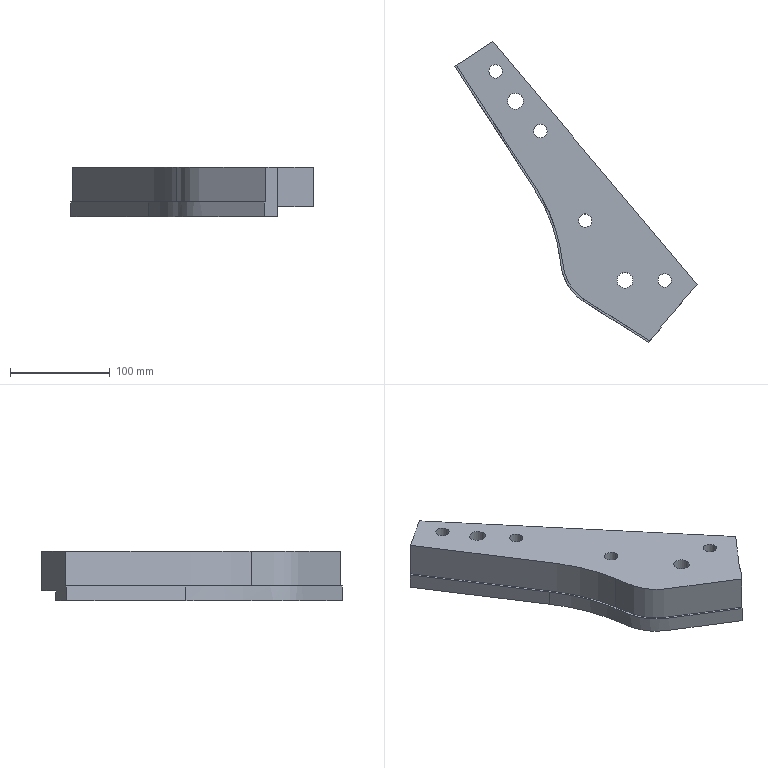Part | NX | features solid 2 | 1 solid | 30 faces | box 243.51 x 301.94 x 50 mm | volume 934799 mm3 | plane 14 | cylinder 10 | spline 6 | commonest cylinder face diameters 13.5 x4 19.5 x4 16 x2